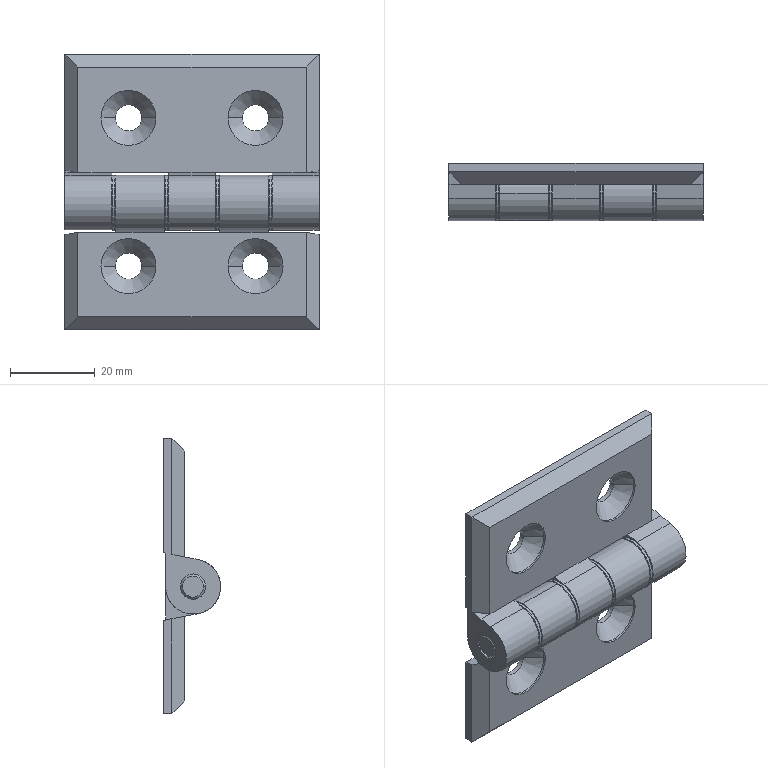Part | STEP file | AKQ41-G-Z-6065 | 3 solids | 168 faces | box 60 x 13.5 x 65 mm | volume 16186 mm3 | plane 68 | cylinder 62 | cone 22 | spline 16 | commonest cylinder face diameters 13 x24 6 x20 10.2 x10 6.2 x8